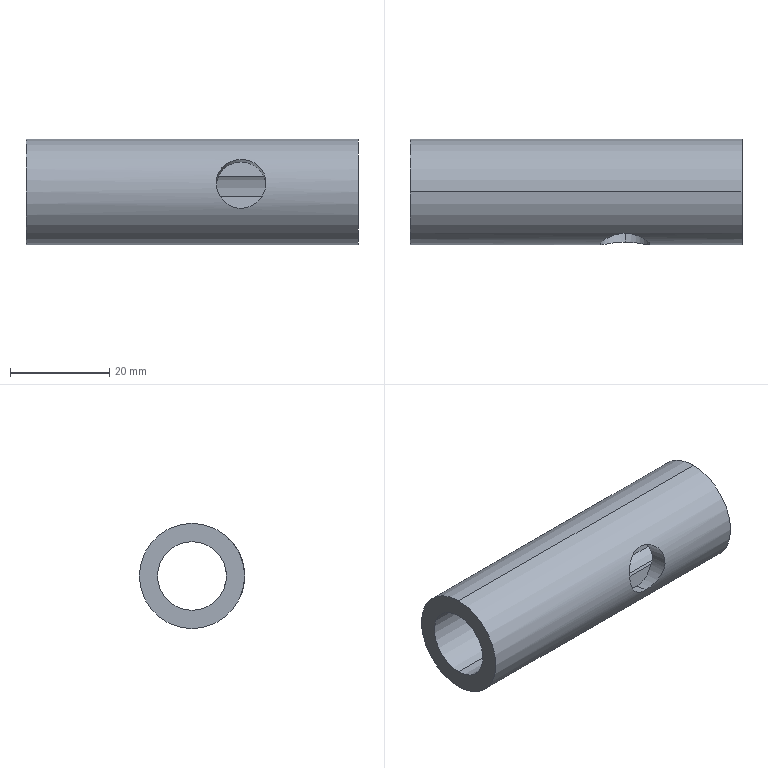Part | SolidWorks | features BaseBody 1, ICE 1 | 1 solid | 10 faces | box 67 x 21.234 x 21.234 mm | volume 13325 mm3 | cylinder 6 | plane 4 | commonest cylinder face diameters 10 x2 13.868 x2 21.234 x2
STEP:
#1=CARTESIAN_POINT('',(394.668,-63.762,10.617));
#2=VERTEX_POINT('',#1);
#3=CARTESIAN_POINT('',(327.668,-63.762,10.617));
#4=VERTEX_POINT('',#3);
#5=CARTESIAN_POINT('',(1067.668,-63.762,10.617));
#6=DIRECTION('',(-1.,0.,0.));
#7=VECTOR('',#6,1000.);
#8=LINE('',#5,#7);
#9=EDGE_CURVE('',#2,#4,#8,.T.);
#10=ORIENTED_EDGE('',*,*,#9,.F.);
#11=CARTESIAN_POINT('',(394.668,-63.762,-10.617));
#12=VERTEX_POINT('',#11);
#13=CARTESIAN_POINT('',(394.668,-63.762,0.));
#14=DIRECTION('',(1.,0.,0.));
#15=DIRECTION('',(0.,0.,-1.));
#16=AXIS2_PLACEMENT_3D('',#13,#14,#15);
#17=CIRCLE('',#16,10.617);
#18=EDGE_CURVE('',#12,#2,#17,.T.);
#19=ORIENTED_EDGE('',*,*,#18,.F.);
#20=CARTESIAN_POINT('',(327.668,-63.762,-10.617));
#21=VERTEX_POINT('',#20);
#22=CARTESIAN_POINT('',(327.668,-63.762,-10.617));
#23=DIRECTION('',(1.,0.,0.));
#24=VECTOR('',#23,1000.);
#25=LINE('',#22,#24);
#26=EDGE_CURVE('',#21,#12,#25,.T.);
#27=ORIENTED_EDGE('',*,*,#26,.F.);
#28=CARTESIAN_POINT('',(327.668,-63.762,0.));
#29=DIRECTION('',(1.,0.,0.));
#30=DIRECTION('',(0.,0.,-1.));
#31=AXIS2_PLACEMENT_3D('',#28,#29,#30);
#32=CIRCLE('',#31,10.617);
#33=EDGE_CURVE('',#21,#4,#32,.T.);
#34=ORIENTED_EDGE('',*,*,#33,.T.);
#35=EDGE_LOOP('',(#10,#19,#27,#34));
#36=FACE_OUTER_BOUND('',#35,.T.);
#37=CARTESIAN_POINT('',(327.668,-63.762,0.));
#38=DIRECTION('',(1.,0.,0.));
#39=DIRECTION('',(0.,0.,-1.));
#40=AXIS2_PLACEMENT_3D('',#37,#38,#39);
#41=CYLINDRICAL_SURFACE('',#40,10.617);
#42=ADVANCED_FACE('',(#36),#41,.T.);
#43=CARTESIAN_POINT('',(371.081,-73.854,-3.298));
#44=VERTEX_POINT('',#43);
#45=CARTESIAN_POINT('',(376.081,-74.218,1.844));
#46=VERTEX_POINT('',#45);
#47=CARTESIAN_POINT('',(371.081,-73.854,-3.298));
#48=CARTESIAN_POINT('',(371.388,-73.854,-3.298));
#49=CARTESIAN_POINT('',(371.707,-73.865,-3.267));
#50=CARTESIAN_POINT('',(372.192,-73.897,-3.166));
#51=CARTESIAN_POINT('',(372.355,-73.91,-3.123));
#52=CARTESIAN_POINT('',(372.599,-73.933,-3.044));
#53=CARTESIAN_POINT('',(372.722,-73.946,-3.002));
#54=CARTESIAN_POINT('',(372.864,-73.962,-2.945));
#55=CARTESIAN_POINT('',(372.935,-73.971,-2.915));
#56=CARTESIAN_POINT('',(372.971,-73.975,-2.9));
#57=CARTESIAN_POINT('',(372.989,-73.978,-2.892));
#58=CARTESIAN_POINT('',(372.996,-73.978,-2.888));
#59=CARTESIAN_POINT('',(373.001,-73.979,-2.886));
#60=CARTESIAN_POINT('',(373.005,-73.98,-2.884));
#61=CARTESIAN_POINT('',(373.189,-74.003,-2.803));
#62=CARTESIAN_POINT('',(373.426,-74.038,-2.684));
#63=CARTESIAN_POINT('',(373.841,-74.104,-2.413));
#64=CARTESIAN_POINT('',(373.988,-74.128,-2.307));
#65=CARTESIAN_POINT('',(374.218,-74.167,-2.12));
#66=CARTESIAN_POINT('',(374.296,-74.18,-2.052));
#67=CARTESIAN_POINT('',(374.415,-74.2,-1.944));
#68=CARTESIAN_POINT('',(374.474,-74.21,-1.887));
#69=CARTESIAN_POINT('',(374.544,-74.222,-1.818));
#70=CARTESIAN_POINT('',(374.574,-74.227,-1.788));
#71=CARTESIAN_POINT('',(374.594,-74.231,-1.767));
#72=CARTESIAN_POINT('',(374.605,-74.233,-1.756));
#73=CARTESIAN_POINT('',(374.904,-74.285,-1.443));
#74=CARTESIAN_POINT('',(375.128,-74.32,-1.137));
#75=CARTESIAN_POINT('',(375.39,-74.354,-0.7131));
#76=CARTESIAN_POINT('',(375.464,-74.363,-0.5772));
#77=CARTESIAN_POINT('',(375.561,-74.371,-0.3845));
#78=CARTESIAN_POINT('',(375.591,-74.374,-0.3221));
#79=CARTESIAN_POINT('',(375.632,-74.376,-0.2316));
#80=CARTESIAN_POINT('',(375.651,-74.377,-0.1871));
#81=CARTESIAN_POINT('',(375.673,-74.378,-0.1365));
#82=CARTESIAN_POINT('',(375.683,-74.378,-0.1116));
#83=CARTESIAN_POINT('',(375.688,-74.378,-0.101));
#84=CARTESIAN_POINT('',(375.691,-74.378,-0.09396));
#85=CARTESIAN_POINT('',(375.692,-74.379,-0.092));
#86=CARTESIAN_POINT('',(375.96,-74.384,0.5614));
#87=CARTESIAN_POINT('',(376.081,-74.327,1.224));
#88=CARTESIAN_POINT('',(376.081,-74.218,1.844));
#89=B_SPLINE_CURVE_WITH_KNOTS('',3,(#47,#48,#49,#50,#51,#52,#53,#54,#55,#56,#57,#58,#59,#60,#61,#62,#63,#64,#65,#66,#67,#68,#69,#70,#71,#72,#73,#74,#75,#76,#77,#78,#79,#80,#81,#82,#83,#84,#85,#86,#87,#88),.UNSPECIFIED.,.F.,.F.,(4,2,2,1,1,1,1,1,2,2,2,2,2,1,1,2,2,2,2,2,1,1,1,2,2,4),(0.,0.125,0.1875,0.2187,0.2344,0.2422,0.2461,0.248,0.249,0.25,0.375,0.4375,0.4687,0.4844,0.4922,0.4961,0.5,0.625,0.6875,0.7187,0.7344,0.7422,0.7461,0.748,0.75,1.),.UNSPECIFIED.);
#90=EDGE_CURVE('',#44,#46,#89,.T.);
#91=ORIENTED_EDGE('',*,*,#90,.F.);
#92=CARTESIAN_POINT('',(366.081,-74.218,1.844));
#93=VERTEX_POINT('',#92);
#94=CARTESIAN_POINT('',(366.081,-74.218,1.844));
#95=CARTESIAN_POINT('',(366.081,-74.272,1.534));
#96=CARTESIAN_POINT('',(366.111,-74.314,1.214));
#97=CARTESIAN_POINT('',(366.206,-74.355,0.7275));
#98=CARTESIAN_POINT('',(366.246,-74.365,0.5645));
#99=CARTESIAN_POINT('',(366.319,-74.374,0.3198));
#100=CARTESIAN_POINT('',(366.359,-74.377,0.1975));
#101=CARTESIAN_POINT('',(366.412,-74.379,0.05512));
#102=CARTESIAN_POINT('',(366.439,-74.379,-0.01596));
#103=CARTESIAN_POINT('',(366.454,-74.379,-0.05146));
#104=CARTESIAN_POINT('',(366.46,-74.379,-0.06667));
#105=CARTESIAN_POINT('',(366.464,-74.379,-0.0768));
#106=CARTESIAN_POINT('',(366.467,-74.379,-0.08343));
#107=CARTESIAN_POINT('',(366.56,-74.377,-0.3113));
#108=CARTESIAN_POINT('',(366.685,-74.366,-0.5716));
#109=CARTESIAN_POINT('',(366.946,-74.331,-0.9957));
#110=CARTESIAN_POINT('',(367.046,-74.317,-1.143));
#111=CARTESIAN_POINT('',(367.217,-74.29,-1.367));
#112=CARTESIAN_POINT('',(367.277,-74.28,-1.443));
#113=CARTESIAN_POINT('',(367.374,-74.264,-1.556));
#114=CARTESIAN_POINT('',(367.424,-74.256,-1.613));
#115=CARTESIAN_POINT('',(367.485,-74.245,-1.68));
#116=CARTESIAN_POINT('',(367.512,-74.241,-1.708));
#117=CARTESIAN_POINT('',(367.53,-74.237,-1.727));
#118=CARTESIAN_POINT('',(367.538,-74.236,-1.736));
#119=CARTESIAN_POINT('',(367.867,-74.179,-2.08));
#120=CARTESIAN_POINT('',(368.183,-74.126,-2.323));
#121=CARTESIAN_POINT('',(368.597,-74.06,-2.594));
#122=CARTESIAN_POINT('',(368.726,-74.04,-2.668));
#123=CARTESIAN_POINT('',(368.901,-74.014,-2.762));
#124=CARTESIAN_POINT('',(368.956,-74.007,-2.79));
#125=CARTESIAN_POINT('',(369.035,-73.996,-2.828));
#126=CARTESIAN_POINT('',(369.073,-73.99,-2.846));
#127=CARTESIAN_POINT('',(369.115,-73.985,-2.866));
#128=CARTESIAN_POINT('',(369.135,-73.982,-2.875));
#129=CARTESIAN_POINT('',(369.145,-73.981,-2.879));
#130=CARTESIAN_POINT('',(369.15,-73.98,-2.881));
#131=CARTESIAN_POINT('',(369.152,-73.98,-2.883));
#132=CARTESIAN_POINT('',(369.153,-73.98,-2.883));
#133=CARTESIAN_POINT('',(369.804,-73.898,-3.173));
#134=CARTESIAN_POINT('',(370.466,-73.854,-3.298));
#135=CARTESIAN_POINT('',(371.081,-73.854,-3.298));
#136=B_SPLINE_CURVE_WITH_KNOTS('',3,(#94,#95,#96,#97,#98,#99,#100,#101,#102,#103,#104,#105,#106,#107,#108,#109,#110,#111,#112,#113,#114,#115,#116,#117,#118,#119,#120,#121,#122,#123,#124,#125,#126,#127,#128,#129,#130,#131,#132,#133,#134,#135),.UNSPECIFIED.,.F.,.F.,(4,2,2,1,1,1,1,2,2,2,2,2,1,1,2,2,2,2,2,1,1,1,1,2,2,4),(0.,0.125,0.1875,0.2187,0.2344,0.2422,0.2461,0.248,0.25,0.375,0.4375,0.4687,0.4844,0.4922,0.4961,0.5,0.625,0.6875,0.7187,0.7344,0.7422,0.7461,0.748,0.749,0.75,1.),.UNSPECIFIED.);
#137=EDGE_CURVE('',#93,#44,#136,.T.);
#138=ORIENTED_EDGE('',*,*,#137,.F.);
#139=CARTESIAN_POINT('',(371.081,-72.117,6.55));
#140=VERTEX_POINT('',#139);
#141=CARTESIAN_POINT('',(371.081,-72.117,6.55));
#142=CARTESIAN_POINT('',(370.773,-72.117,6.55));
#143=CARTESIAN_POINT('',(370.455,-72.138,6.525));
#144=CARTESIAN_POINT('',(369.97,-72.203,6.441));
#145=CARTESIAN_POINT('',(369.807,-72.23,6.406));
#146=CARTESIAN_POINT('',(369.562,-72.279,6.34));
#147=CARTESIAN_POINT('',(369.44,-72.305,6.304));
#148=CARTESIAN_POINT('',(369.297,-72.34,6.256));
#149=CARTESIAN_POINT('',(369.226,-72.358,6.231));
#150=CARTESIAN_POINT('',(369.191,-72.368,6.218));
#151=CARTESIAN_POINT('',(369.173,-72.372,6.211));
#152=CARTESIAN_POINT('',(369.165,-72.374,6.209));
#153=CARTESIAN_POINT('',(369.16,-72.376,6.207));
#154=CARTESIAN_POINT('',(369.157,-72.377,6.205));
#155=CARTESIAN_POINT('',(368.973,-72.427,6.136));
#156=CARTESIAN_POINT('',(368.735,-72.501,6.037));
#157=CARTESIAN_POINT('',(368.321,-72.655,5.805));
#158=CARTESIAN_POINT('',(368.173,-72.714,5.714));
#159=CARTESIAN_POINT('',(367.943,-72.814,5.551));
#160=CARTESIAN_POINT('',(367.865,-72.85,5.492));
#161=CARTESIAN_POINT('',(367.747,-72.906,5.397));
#162=CARTESIAN_POINT('',(367.688,-72.935,5.347));
#163=CARTESIAN_POINT('',(367.618,-72.97,5.286));
#164=CARTESIAN_POINT('',(367.588,-72.985,5.259));
#165=CARTESIAN_POINT('',(367.568,-72.995,5.241));
#166=CARTESIAN_POINT('',(367.557,-73.001,5.231));
#167=CARTESIAN_POINT('',(367.257,-73.157,4.955));
#168=CARTESIAN_POINT('',(367.033,-73.294,4.68));
#169=CARTESIAN_POINT('',(366.772,-73.471,4.293));
#170=CARTESIAN_POINT('',(366.697,-73.526,4.168));
#171=CARTESIAN_POINT('',(366.601,-73.6,3.99));
#172=CARTESIAN_POINT('',(366.571,-73.624,3.932));
#173=CARTESIAN_POINT('',(366.53,-73.657,3.848));
#174=CARTESIAN_POINT('',(366.51,-73.673,3.806));
#175=CARTESIAN_POINT('',(366.489,-73.691,3.759));
#176=CARTESIAN_POINT('',(366.478,-73.7,3.736));
#177=CARTESIAN_POINT('',(366.474,-73.704,3.726));
#178=CARTESIAN_POINT('',(366.471,-73.706,3.719));
#179=CARTESIAN_POINT('',(366.47,-73.707,3.718));
#180=CARTESIAN_POINT('',(366.201,-73.935,3.105));
#181=CARTESIAN_POINT('',(366.081,-74.108,2.463));
#182=CARTESIAN_POINT('',(366.081,-74.218,1.844));
#183=B_SPLINE_CURVE_WITH_KNOTS('',3,(#141,#142,#143,#144,#145,#146,#147,#148,#149,#150,#151,#152,#153,#154,#155,#156,#157,#158,#159,#160,#161,#162,#163,#164,#165,#166,#167,#168,#169,#170,#171,#172,#173,#174,#175,#176,#177,#178,#179,#180,#181,#182),.UNSPECIFIED.,.F.,.F.,(4,2,2,1,1,1,1,1,2,2,2,2,2,1,1,2,2,2,2,2,1,1,1,2,2,4),(0.,0.125,0.1875,0.2187,0.2344,0.2422,0.2461,0.248,0.249,0.25,0.375,0.4375,0.4687,0.4844,0.4922,0.4961,0.5,0.625,0.6875,0.7188,0.7344,0.7422,0.7461,0.748,0.75,1.),.UNSPECIFIED.);
#184=EDGE_CURVE('',#140,#93,#183,.T.);
#185=ORIENTED_EDGE('',*,*,#184,.F.);
#186=CARTESIAN_POINT('',(376.081,-74.218,1.844));
#187=CARTESIAN_POINT('',(376.081,-74.163,2.153));
#188=CARTESIAN_POINT('',(376.051,-74.092,2.468));
#189=CARTESIAN_POINT('',(375.956,-73.965,2.939));
#190=CARTESIAN_POINT('',(375.916,-73.918,3.096));
#191=CARTESIAN_POINT('',(375.842,-73.844,3.329));
#192=CARTESIAN_POINT('',(375.802,-73.805,3.445));
#193=CARTESIAN_POINT('',(375.75,-73.757,3.579));
#194=CARTESIAN_POINT('',(375.722,-73.733,3.646));
#195=CARTESIAN_POINT('',(375.708,-73.721,3.68));
#196=CARTESIAN_POINT('',(375.702,-73.716,3.694));
#197=CARTESIAN_POINT('',(375.698,-73.712,3.703));
#198=CARTESIAN_POINT('',(375.695,-73.71,3.71));
#199=CARTESIAN_POINT('',(375.601,-73.63,3.923));
#200=CARTESIAN_POINT('',(375.477,-73.531,4.164));
#201=CARTESIAN_POINT('',(375.216,-73.353,4.551));
#202=CARTESIAN_POINT('',(375.116,-73.289,4.684));
#203=CARTESIAN_POINT('',(374.945,-73.187,4.885));
#204=CARTESIAN_POINT('',(374.884,-73.152,4.953));
#205=CARTESIAN_POINT('',(374.787,-73.098,5.054));
#206=CARTESIAN_POINT('',(374.737,-73.071,5.105));
#207=CARTESIAN_POINT('',(374.676,-73.038,5.164));
#208=CARTESIAN_POINT('',(374.65,-73.024,5.189));
#209=CARTESIAN_POINT('',(374.632,-73.015,5.206));
#210=CARTESIAN_POINT('',(374.624,-73.011,5.214));
#211=CARTESIAN_POINT('',(374.294,-72.839,5.517));
#212=CARTESIAN_POINT('',(373.979,-72.707,5.728));
#213=CARTESIAN_POINT('',(373.564,-72.552,5.96));
#214=CARTESIAN_POINT('',(373.436,-72.508,6.023));
#215=CARTESIAN_POINT('',(373.261,-72.452,6.102));
#216=CARTESIAN_POINT('',(373.205,-72.434,6.126));
#217=CARTESIAN_POINT('',(373.127,-72.411,6.158));
#218=CARTESIAN_POINT('',(373.089,-72.4,6.173));
#219=CARTESIAN_POINT('',(373.047,-72.388,6.189));
#220=CARTESIAN_POINT('',(373.026,-72.383,6.197));
#221=CARTESIAN_POINT('',(373.016,-72.38,6.201));
#222=CARTESIAN_POINT('',(373.012,-72.379,6.203));
#223=CARTESIAN_POINT('',(373.009,-72.378,6.204));
#224=CARTESIAN_POINT('',(373.009,-72.378,6.204));
#225=CARTESIAN_POINT('',(372.358,-72.202,6.449));
#226=CARTESIAN_POINT('',(371.696,-72.117,6.55));
#227=CARTESIAN_POINT('',(371.081,-72.117,6.55));
#228=B_SPLINE_CURVE_WITH_KNOTS('',3,(#186,#187,#188,#189,#190,#191,#192,#193,#194,#195,#196,#197,#198,#199,#200,#201,#202,#203,#204,#205,#206,#207,#208,#209,#210,#211,#212,#213,#214,#215,#216,#217,#218,#219,#220,#221,#222,#223,#224,#225,#226,#227),.UNSPECIFIED.,.F.,.F.,(4,2,2,1,1,1,1,2,2,2,2,2,1,1,2,2,2,2,2,1,1,1,1,2,2,4),(0.,0.125,0.1875,0.2188,0.2344,0.2422,0.2461,0.248,0.25,0.375,0.4375,0.4688,0.4844,0.4922,0.4961,0.5,0.625,0.6875,0.7188,0.7344,0.7422,0.7461,0.748,0.749,0.75,1.),.UNSPECIFIED.);
#229=EDGE_CURVE('',#46,#140,#228,.T.);
#230=ORIENTED_EDGE('',*,*,#229,.F.);
#231=EDGE_LOOP('',(#91,#138,#185,#230));
#232=FACE_BOUND('',#231,.T.);
#233=ORIENTED_EDGE('',*,*,#26,.T.);
#234=CARTESIAN_POINT('',(394.668,-63.762,0.));
#235=DIRECTION('',(1.,0.,0.));
#236=DIRECTION('',(0.,0.,-1.));
#237=AXIS2_PLACEMENT_3D('',#234,#235,#236);
#238=CIRCLE('',#237,10.617);
#239=EDGE_CURVE('',#2,#12,#238,.T.);
#240=ORIENTED_EDGE('',*,*,#239,.F.);
#241=ORIENTED_EDGE('',*,*,#9,.T.);
#242=CARTESIAN_POINT('',(327.668,-63.762,0.));
#243=DIRECTION('',(1.,0.,0.));
#244=DIRECTION('',(0.,0.,1.));
#245=AXIS2_PLACEMENT_3D('',#242,#243,#244);
#246=CIRCLE('',#245,10.617);
#247=EDGE_CURVE('',#4,#21,#246,.T.);
#248=ORIENTED_EDGE('',*,*,#247,.T.);
#249=EDGE_LOOP('',(#233,#240,#241,#248));
#250=FACE_OUTER_BOUND('',#249,.T.);
#251=CARTESIAN_POINT('',(327.668,-63.762,0.));
#252=DIRECTION('',(1.,0.,0.));
#253=DIRECTION('',(0.,0.,-1.));
#254=AXIS2_PLACEMENT_3D('',#251,#252,#253);
#255=CYLINDRICAL_SURFACE('',#254,10.617);
#256=ADVANCED_FACE('',(#232,#250),#255,.T.);
#257=CARTESIAN_POINT('',(375.631,-69.918,3.19));
#258=VERTEX_POINT('',#257);
#259=CARTESIAN_POINT('',(375.631,-70.638,-0.8921));
#260=VERTEX_POINT('',#259);
#261=CARTESIAN_POINT('',(375.631,-69.918,3.19));
#262=CARTESIAN_POINT('',(375.938,-70.244,2.563));
#263=CARTESIAN_POINT('',(376.081,-70.472,1.877));
#264=CARTESIAN_POINT('',(376.081,-70.709,0.5312));
#265=CARTESIAN_POINT('',(375.938,-70.729,-0.1908));
#266=CARTESIAN_POINT('',(375.631,-70.638,-0.8921));
#267=B_SPLINE_CURVE_WITH_KNOTS('',3,(#261,#262,#263,#264,#265,#266),.UNSPECIFIED.,.F.,.F.,(4,2,4),(0.,0.5,1.),.UNSPECIFIED.);
#268=EDGE_CURVE('',#258,#260,#267,.T.);
#269=ORIENTED_EDGE('',*,*,#268,.F.);
#270=CARTESIAN_POINT('',(366.531,-69.918,3.19));
#271=VERTEX_POINT('',#270);
#272=CARTESIAN_POINT('',(366.531,-69.918,3.19));
#273=DIRECTION('',(1.,0.,0.));
#274=VECTOR('',#273,1000.);
#275=LINE('',#272,#274);
#276=EDGE_CURVE('',#271,#258,#275,.T.);
#277=ORIENTED_EDGE('',*,*,#276,.F.);
#278=CARTESIAN_POINT('',(366.531,-70.638,-0.8921));
#279=VERTEX_POINT('',#278);
#280=CARTESIAN_POINT('',(366.531,-70.638,-0.8921));
#281=CARTESIAN_POINT('',(366.223,-70.729,-0.191));
#282=CARTESIAN_POINT('',(366.081,-70.709,0.5312));
#283=CARTESIAN_POINT('',(366.081,-70.472,1.877));
#284=CARTESIAN_POINT('',(366.223,-70.244,2.562));
#285=CARTESIAN_POINT('',(366.531,-69.918,3.19));
#286=B_SPLINE_CURVE_WITH_KNOTS('',3,(#280,#281,#282,#283,#284,#285),.UNSPECIFIED.,.F.,.F.,(4,2,4),(0.,0.5,1.),.UNSPECIFIED.);
#287=EDGE_CURVE('',#279,#271,#286,.T.);
#288=ORIENTED_EDGE('',*,*,#287,.F.);
#289=CARTESIAN_POINT('',(375.631,-70.638,-0.8921));
#290=DIRECTION('',(-1.,0.,0.));
#291=VECTOR('',#290,1000.);
#292=LINE('',#289,#291);
#293=EDGE_CURVE('',#260,#279,#292,.T.);
#294=ORIENTED_EDGE('',*,*,#293,.F.);
#295=EDGE_LOOP('',(#269,#277,#288,#294));
#296=FACE_BOUND('',#295,.T.);
#297=CARTESIAN_POINT('',(394.668,-63.762,-6.934));
#298=VERTEX_POINT('',#297);
#299=CARTESIAN_POINT('',(394.668,-63.762,6.934));
#300=VERTEX_POINT('',#299);
#301=CARTESIAN_POINT('',(394.668,-63.762,0.));
#302=DIRECTION('',(-1.,0.,0.));
#303=DIRECTION('',(0.,0.,-1.));
#304=AXIS2_PLACEMENT_3D('',#301,#302,#303);
#305=CIRCLE('',#304,6.934);
#306=EDGE_CURVE('',#298,#300,#305,.T.);
#307=ORIENTED_EDGE('',*,*,#306,.F.);
#308=CARTESIAN_POINT('',(327.668,-63.762,-6.934));
#309=VERTEX_POINT('',#308);
#310=CARTESIAN_POINT('',(327.668,-63.762,-6.934));
#311=DIRECTION('',(1.,0.,0.));
#312=VECTOR('',#311,1000.);
#313=LINE('',#310,#312);
#314=EDGE_CURVE('',#309,#298,#313,.T.);
#315=ORIENTED_EDGE('',*,*,#314,.F.);
#316=CARTESIAN_POINT('',(327.668,-63.762,6.934));
#317=VERTEX_POINT('',#316);
#318=CARTESIAN_POINT('',(327.668,-63.762,0.));
#319=DIRECTION('',(-1.,0.,0.));
#320=DIRECTION('',(0.,0.,-1.));
#321=AXIS2_PLACEMENT_3D('',#318,#319,#320);
#322=CIRCLE('',#321,6.934);
#323=EDGE_CURVE('',#309,#317,#322,.T.);
#324=ORIENTED_EDGE('',*,*,#323,.T.);
#325=CARTESIAN_POINT('',(1067.668,-63.762,6.934));
#326=DIRECTION('',(-1.,0.,0.));
#327=VECTOR('',#326,1000.);
#328=LINE('',#325,#327);
#329=EDGE_CURVE('',#300,#317,#328,.T.);
#330=ORIENTED_EDGE('',*,*,#329,.F.);
#331=EDGE_LOOP('',(#307,#315,#324,#330));
#332=FACE_OUTER_BOUND('',#331,.T.);
#333=CARTESIAN_POINT('',(327.668,-63.762,0.));
#334=DIRECTION('',(1.,0.,0.));
#335=DIRECTION('',(0.,0.,-1.));
#336=AXIS2_PLACEMENT_3D('',#333,#334,#335);
#337=CYLINDRICAL_SURFACE('',#336,6.934);
#338=ADVANCED_FACE('',(#296,#332),#337,.F.);
#339=CARTESIAN_POINT('',(394.668,-63.762,0.));
#340=DIRECTION('',(-1.,0.,0.));
#341=DIRECTION('',(0.,0.,-1.));
#342=AXIS2_PLACEMENT_3D('',#339,#340,#341);
#343=CIRCLE('',#342,6.934);
#344=EDGE_CURVE('',#300,#298,#343,.T.);
#345=ORIENTED_EDGE('',*,*,#344,.F.);
#346=ORIENTED_EDGE('',*,*,#329,.T.);
#347=CARTESIAN_POINT('',(327.668,-63.762,0.));
#348=DIRECTION('',(-1.,0.,0.));
#349=DIRECTION('',(0.,0.,1.));
#350=AXIS2_PLACEMENT_3D('',#347,#348,#349);
#351=CIRCLE('',#350,6.934);
#352=EDGE_CURVE('',#317,#309,#351,.T.);
#353=ORIENTED_EDGE('',*,*,#352,.T.);
#354=ORIENTED_EDGE('',*,*,#314,.T.);
#355=EDGE_LOOP('',(#345,#346,#353,#354));
#356=FACE_OUTER_BOUND('',#355,.T.);
#357=CARTESIAN_POINT('',(327.668,-63.762,0.));
#358=DIRECTION('',(1.,0.,0.));
#359=DIRECTION('',(0.,0.,-1.));
#360=AXIS2_PLACEMENT_3D('',#357,#358,#359);
#361=CYLINDRICAL_SURFACE('',#360,6.934);
#362=ADVANCED_FACE('',(#356),#361,.F.);
#363=ORIENTED_EDGE('',*,*,#323,.F.);
#364=ORIENTED_EDGE('',*,*,#352,.F.);
#365=EDGE_LOOP('',(#363,#364));
#366=FACE_BOUND('',#365,.T.);
#367=ORIENTED_EDGE('',*,*,#33,.F.);
#368=ORIENTED_EDGE('',*,*,#247,.F.);
#369=EDGE_LOOP('',(#367,#368));
#370=FACE_OUTER_BOUND('',#369,.T.);
#371=CARTESIAN_POINT('',(327.668,-63.762,0.));
#372=DIRECTION('',(-1.,0.,0.));
#373=DIRECTION('',(0.,0.,1.));
#374=AXIS2_PLACEMENT_3D('',#371,#372,#373);
#375=PLANE('',#374);
#376=ADVANCED_FACE('',(#366,#370),#375,.T.);
#377=ORIENTED_EDGE('',*,*,#276,.T.);
#378=CARTESIAN_POINT('',(371.081,-69.41,6.073));
#379=VERTEX_POINT('',#378);
#380=CARTESIAN_POINT('',(371.081,-70.278,1.149));
#381=DIRECTION('',(0.,0.9848,-0.1736));
#382=DIRECTION('',(0.,0.1736,0.9848));
#383=AXIS2_PLACEMENT_3D('',#380,#381,#382);
#384=CIRCLE('',#383,5.);
#385=EDGE_CURVE('',#379,#258,#384,.T.);
#386=ORIENTED_EDGE('',*,*,#385,.F.);
#387=CARTESIAN_POINT('',(371.081,-70.278,1.149));
#388=DIRECTION('',(0.,0.9848,-0.1736));
#389=DIRECTION('',(-0.91,0.07198,0.4082));
#390=AXIS2_PLACEMENT_3D('',#387,#388,#389);
#391=CIRCLE('',#390,5.);
#392=EDGE_CURVE('',#271,#379,#391,.T.);
#393=ORIENTED_EDGE('',*,*,#392,.F.);
#394=EDGE_LOOP('',(#377,#386,#393));
#395=FACE_OUTER_BOUND('',#394,.T.);
#396=CARTESIAN_POINT('',(371.081,-70.278,1.149));
#397=DIRECTION('',(0.,-0.9848,0.1736));
#398=DIRECTION('',(-1.,0.,0.));
#399=AXIS2_PLACEMENT_3D('',#396,#397,#398);
#400=PLANE('',#399);
#401=ADVANCED_FACE('',(#395),#400,.T.);
#402=ORIENTED_EDGE('',*,*,#90,.T.);
#403=ORIENTED_EDGE('',*,*,#229,.T.);
#404=CARTESIAN_POINT('',(371.081,-69.41,6.073));
#405=DIRECTION('',(0.,-0.9848,0.1736));
#406=VECTOR('',#405,1000.);
#407=LINE('',#404,#406);
#408=EDGE_CURVE('',#379,#140,#407,.T.);
#409=ORIENTED_EDGE('',*,*,#408,.F.);
#410=ORIENTED_EDGE('',*,*,#385,.T.);
#411=ORIENTED_EDGE('',*,*,#268,.T.);
#412=CARTESIAN_POINT('',(371.081,-71.147,-3.775));
#413=VERTEX_POINT('',#412);
#414=CARTESIAN_POINT('',(371.081,-70.278,1.149));
#415=DIRECTION('',(0.,-0.9848,0.1736));
#416=DIRECTION('',(0.,-0.1736,-0.9848));
#417=AXIS2_PLACEMENT_3D('',#414,#415,#416);
#418=CIRCLE('',#417,5.);
#419=EDGE_CURVE('',#413,#260,#418,.T.);
#420=ORIENTED_EDGE('',*,*,#419,.F.);
#421=CARTESIAN_POINT('',(371.081,-73.854,-3.298));
#422=DIRECTION('',(0.,0.9848,-0.1736));
#423=VECTOR('',#422,1000.);
#424=LINE('',#421,#423);
#425=EDGE_CURVE('',#44,#413,#424,.T.);
#426=ORIENTED_EDGE('',*,*,#425,.F.);
#427=EDGE_LOOP('',(#402,#403,#409,#410,#411,#420,#426));
#428=FACE_OUTER_BOUND('',#427,.T.);
#429=CARTESIAN_POINT('',(371.081,-74.218,1.844));
#430=DIRECTION('',(0.,0.9848,-0.1736));
#431=DIRECTION('',(0.,0.1736,0.9848));
#432=AXIS2_PLACEMENT_3D('',#429,#430,#431);
#433=CYLINDRICAL_SURFACE('',#432,5.);
#434=ADVANCED_FACE('',(#428),#433,.F.);
#435=ORIENTED_EDGE('',*,*,#137,.T.);
#436=ORIENTED_EDGE('',*,*,#425,.T.);
#437=CARTESIAN_POINT('',(371.081,-70.278,1.149));
#438=DIRECTION('',(0.,-0.9848,0.1736));
#439=DIRECTION('',(-0.91,-0.07198,-0.4082));
#440=AXIS2_PLACEMENT_3D('',#437,#438,#439);
#441=CIRCLE('',#440,5.);
#442=EDGE_CURVE('',#279,#413,#441,.T.);
#443=ORIENTED_EDGE('',*,*,#442,.F.);
#444=ORIENTED_EDGE('',*,*,#287,.T.);
#445=ORIENTED_EDGE('',*,*,#392,.T.);
#446=ORIENTED_EDGE('',*,*,#408,.T.);
#447=ORIENTED_EDGE('',*,*,#184,.T.);
#448=EDGE_LOOP('',(#435,#436,#443,#444,#445,#446,#447));
#449=FACE_OUTER_BOUND('',#448,.T.);
#450=CARTESIAN_POINT('',(371.081,-74.218,1.844));
#451=DIRECTION('',(0.,0.9848,-0.1736));
#452=DIRECTION('',(0.,0.1736,0.9848));
#453=AXIS2_PLACEMENT_3D('',#450,#451,#452);
#454=CYLINDRICAL_SURFACE('',#453,5.);
#455=ADVANCED_FACE('',(#449),#454,.F.);
#456=ORIENTED_EDGE('',*,*,#293,.T.);
#457=ORIENTED_EDGE('',*,*,#442,.T.);
#458=ORIENTED_EDGE('',*,*,#419,.T.);
#459=EDGE_LOOP('',(#456,#457,#458));
#460=FACE_OUTER_BOUND('',#459,.T.);
#461=CARTESIAN_POINT('',(371.081,-70.278,1.149));
#462=DIRECTION('',(0.,-0.9848,0.1736));
#463=DIRECTION('',(-1.,0.,0.));
#464=AXIS2_PLACEMENT_3D('',#461,#462,#463);
#465=PLANE('',#464);
#466=ADVANCED_FACE('',(#460),#465,.T.);
#467=ORIENTED_EDGE('',*,*,#18,.T.);
#468=ORIENTED_EDGE('',*,*,#239,.T.);
#469=EDGE_LOOP('',(#467,#468));
#470=FACE_OUTER_BOUND('',#469,.T.);
#471=ORIENTED_EDGE('',*,*,#306,.T.);
#472=ORIENTED_EDGE('',*,*,#344,.T.);
#473=EDGE_LOOP('',(#471,#472));
#474=FACE_BOUND('',#473,.T.);
#475=CARTESIAN_POINT('',(394.668,-63.762,0.));
#476=DIRECTION('',(1.,0.,0.));
#477=DIRECTION('',(0.,0.,-1.));
#478=AXIS2_PLACEMENT_3D('',#475,#476,#477);
#479=PLANE('',#478);
#480=ADVANCED_FACE('',(#470,#474),#479,.T.);
#481=CLOSED_SHELL('',(#42,#256,#338,#362,#376,#401,#434,#455,#466,#480));
#482=MANIFOLD_SOLID_BREP('',#481);
#483=CARTESIAN_POINT('',(0.,0.,0.));
#484=DIRECTION('',(0.,0.,1.));
#485=DIRECTION('',(1.,0.,0.));
#486=AXIS2_PLACEMENT_3D('',#483,#484,#485);
#487=(LENGTH_UNIT()NAMED_UNIT(*)SI_UNIT(.MILLI.,.METRE.));
#488=UNCERTAINTY_MEASURE_WITH_UNIT(LENGTH_MEASURE(0.00001),#487,'','');
#489=(NAMED_UNIT(*)PLANE_ANGLE_UNIT()SI_UNIT($,.RADIAN.));
#490=(NAMED_UNIT(*)SI_UNIT($,.STERADIAN.)SOLID_ANGLE_UNIT());
#491=(GEOMETRIC_REPRESENTATION_CONTEXT(3)GLOBAL_UNCERTAINTY_ASSIGNED_CONTEXT((#488))GLOBAL_UNIT_ASSIGNED_CONTEXT((#487,#489,#490))REPRESENTATION_CONTEXT('',''));
#492=ADVANCED_BREP_SHAPE_REPRESENTATION('',(#482,#486),#491);